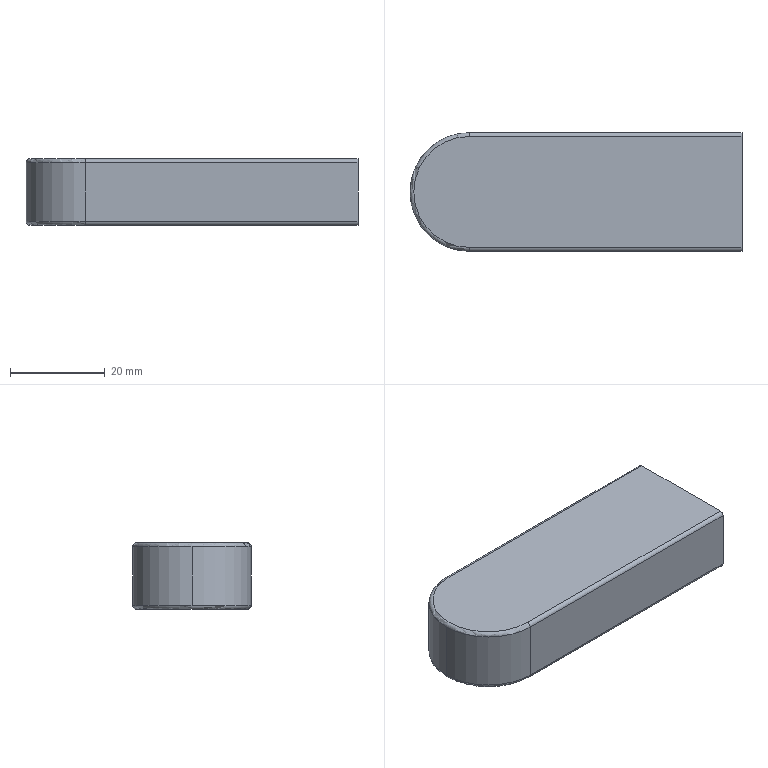Part | SolidWorks | features Extrusion 1, Fillet 1 | 1 solid | 13 faces | box 70 x 25 x 14 mm | volume 23519 mm3 | cylinder 6 | plane 5 | torus 2 | commonest cylinder face diameters 1.6 x4 25 x2
STEP:
#1=CARTESIAN_POINT('',(-9.,-12.5,13.2));
#2=VERTEX_POINT('',#1);
#3=CARTESIAN_POINT('',(-21.5,0.,13.2));
#4=VERTEX_POINT('',#3);
#5=CARTESIAN_POINT('',(-9.,0.,13.2));
#6=DIRECTION('',(0.,0.,-1.));
#7=DIRECTION('',(1.,0.,0.));
#8=AXIS2_PLACEMENT_3D('',#5,#6,#7);
#9=CIRCLE('',#8,12.5);
#10=EDGE_CURVE('',#2,#4,#9,.T.);
#11=ORIENTED_EDGE('',*,*,#10,.T.);
#12=CARTESIAN_POINT('',(-21.5,0.,0.8));
#13=VERTEX_POINT('',#12);
#14=CARTESIAN_POINT('',(-21.5,0.,14.));
#15=DIRECTION('',(0.,0.,-1.));
#16=VECTOR('',#15,1000.);
#17=LINE('',#14,#16);
#18=EDGE_CURVE('',#4,#13,#17,.T.);
#19=ORIENTED_EDGE('',*,*,#18,.T.);
#20=CARTESIAN_POINT('',(-9.,-12.5,0.8));
#21=VERTEX_POINT('',#20);
#22=CARTESIAN_POINT('',(-9.,0.,0.8));
#23=DIRECTION('',(0.,0.,1.));
#24=DIRECTION('',(1.,0.,0.));
#25=AXIS2_PLACEMENT_3D('',#22,#23,#24);
#26=CIRCLE('',#25,12.5);
#27=EDGE_CURVE('',#13,#21,#26,.T.);
#28=ORIENTED_EDGE('',*,*,#27,.T.);
#29=CARTESIAN_POINT('',(-9.,-12.5,14.));
#30=DIRECTION('',(0.,0.,-1.));
#31=VECTOR('',#30,1000.);
#32=LINE('',#29,#31);
#33=EDGE_CURVE('',#2,#21,#32,.T.);
#34=ORIENTED_EDGE('',*,*,#33,.F.);
#35=EDGE_LOOP('',(#11,#19,#28,#34));
#36=FACE_OUTER_BOUND('',#35,.T.);
#37=CARTESIAN_POINT('',(-9.,0.,14.));
#38=DIRECTION('',(0.,0.,-1.));
#39=DIRECTION('',(-1.,0.,0.));
#40=AXIS2_PLACEMENT_3D('',#37,#38,#39);
#41=CYLINDRICAL_SURFACE('',#40,12.5);
#42=ADVANCED_FACE('',(#36),#41,.T.);
#43=CARTESIAN_POINT('',(48.5,-11.7,14.));
#44=VERTEX_POINT('',#43);
#45=CARTESIAN_POINT('',(48.5,11.7,14.));
#46=VERTEX_POINT('',#45);
#47=CARTESIAN_POINT('',(48.5,12.5,14.));
#48=DIRECTION('',(0.,1.,0.));
#49=VECTOR('',#48,1000.);
#50=LINE('',#47,#49);
#51=EDGE_CURVE('',#44,#46,#50,.T.);
#52=ORIENTED_EDGE('',*,*,#51,.F.);
#53=CARTESIAN_POINT('',(48.5,-12.5,13.2));
#54=VERTEX_POINT('',#53);
#55=CARTESIAN_POINT('',(48.5,-11.7,13.2));
#56=DIRECTION('',(1.,0.,0.));
#57=DIRECTION('',(0.,0.,1.));
#58=AXIS2_PLACEMENT_3D('',#55,#56,#57);
#59=CIRCLE('',#58,0.8);
#60=EDGE_CURVE('',#44,#54,#59,.T.);
#61=ORIENTED_EDGE('',*,*,#60,.T.);
#62=CARTESIAN_POINT('',(48.5,-12.5,0.8));
#63=VERTEX_POINT('',#62);
#64=CARTESIAN_POINT('',(48.5,-12.5,14.));
#65=DIRECTION('',(0.,0.,-1.));
#66=VECTOR('',#65,1000.);
#67=LINE('',#64,#66);
#68=EDGE_CURVE('',#54,#63,#67,.T.);
#69=ORIENTED_EDGE('',*,*,#68,.T.);
#70=CARTESIAN_POINT('',(48.5,-11.7,0.));
#71=VERTEX_POINT('',#70);
#72=CARTESIAN_POINT('',(48.5,-11.7,0.8));
#73=DIRECTION('',(1.,0.,0.));
#74=DIRECTION('',(0.,0.,1.));
#75=AXIS2_PLACEMENT_3D('',#72,#73,#74);
#76=CIRCLE('',#75,0.8);
#77=EDGE_CURVE('',#63,#71,#76,.T.);
#78=ORIENTED_EDGE('',*,*,#77,.T.);
#79=CARTESIAN_POINT('',(48.5,11.7,0.));
#80=VERTEX_POINT('',#79);
#81=CARTESIAN_POINT('',(48.5,12.5,0.));
#82=DIRECTION('',(0.,1.,0.));
#83=VECTOR('',#82,1000.);
#84=LINE('',#81,#83);
#85=EDGE_CURVE('',#71,#80,#84,.T.);
#86=ORIENTED_EDGE('',*,*,#85,.T.);
#87=CARTESIAN_POINT('',(48.5,12.5,0.8));
#88=VERTEX_POINT('',#87);
#89=CARTESIAN_POINT('',(48.5,11.7,0.8));
#90=DIRECTION('',(1.,0.,0.));
#91=DIRECTION('',(0.,0.,1.));
#92=AXIS2_PLACEMENT_3D('',#89,#90,#91);
#93=CIRCLE('',#92,0.8);
#94=EDGE_CURVE('',#80,#88,#93,.T.);
#95=ORIENTED_EDGE('',*,*,#94,.T.);
#96=CARTESIAN_POINT('',(48.5,12.5,13.2));
#97=VERTEX_POINT('',#96);
#98=CARTESIAN_POINT('',(48.5,12.5,14.));
#99=DIRECTION('',(0.,0.,-1.));
#100=VECTOR('',#99,1000.);
#101=LINE('',#98,#100);
#102=EDGE_CURVE('',#97,#88,#101,.T.);
#103=ORIENTED_EDGE('',*,*,#102,.F.);
#104=CARTESIAN_POINT('',(48.5,11.7,13.2));
#105=DIRECTION('',(1.,0.,0.));
#106=DIRECTION('',(0.,0.,1.));
#107=AXIS2_PLACEMENT_3D('',#104,#105,#106);
#108=CIRCLE('',#107,0.8);
#109=EDGE_CURVE('',#97,#46,#108,.T.);
#110=ORIENTED_EDGE('',*,*,#109,.T.);
#111=EDGE_LOOP('',(#52,#61,#69,#78,#86,#95,#103,#110));
#112=FACE_OUTER_BOUND('',#111,.T.);
#113=CARTESIAN_POINT('',(48.5,12.5,14.));
#114=DIRECTION('',(-1.,0.,0.));
#115=DIRECTION('',(0.,0.,1.));
#116=AXIS2_PLACEMENT_3D('',#113,#114,#115);
#117=PLANE('',#116);
#118=ADVANCED_FACE('',(#112),#117,.F.);
#119=CARTESIAN_POINT('',(-9.,12.5,13.2));
#120=VERTEX_POINT('',#119);
#121=CARTESIAN_POINT('',(-9.,12.5,0.8));
#122=VERTEX_POINT('',#121);
#123=CARTESIAN_POINT('',(-9.,12.5,14.));
#124=DIRECTION('',(0.,0.,-1.));
#125=VECTOR('',#124,1000.);
#126=LINE('',#123,#125);
#127=EDGE_CURVE('',#120,#122,#126,.T.);
#128=ORIENTED_EDGE('',*,*,#127,.F.);
#129=CARTESIAN_POINT('',(48.5,12.5,13.2));
#130=DIRECTION('',(1.,0.,0.));
#131=VECTOR('',#130,1000.);
#132=LINE('',#129,#131);
#133=EDGE_CURVE('',#120,#97,#132,.T.);
#134=ORIENTED_EDGE('',*,*,#133,.T.);
#135=ORIENTED_EDGE('',*,*,#102,.T.);
#136=CARTESIAN_POINT('',(-9.,12.5,0.8));
#137=DIRECTION('',(-1.,0.,0.));
#138=VECTOR('',#137,1000.);
#139=LINE('',#136,#138);
#140=EDGE_CURVE('',#88,#122,#139,.T.);
#141=ORIENTED_EDGE('',*,*,#140,.T.);
#142=EDGE_LOOP('',(#128,#134,#135,#141));
#143=FACE_OUTER_BOUND('',#142,.T.);
#144=CARTESIAN_POINT('',(-9.,12.5,14.));
#145=DIRECTION('',(0.,-1.,0.));
#146=DIRECTION('',(0.,0.,-1.));
#147=AXIS2_PLACEMENT_3D('',#144,#145,#146);
#148=PLANE('',#147);
#149=ADVANCED_FACE('',(#143),#148,.F.);
#150=ORIENTED_EDGE('',*,*,#18,.F.);
#151=CARTESIAN_POINT('',(-9.,0.,13.2));
#152=DIRECTION('',(0.,0.,-1.));
#153=DIRECTION('',(1.,0.,0.));
#154=AXIS2_PLACEMENT_3D('',#151,#152,#153);
#155=CIRCLE('',#154,12.5);
#156=EDGE_CURVE('',#4,#120,#155,.T.);
#157=ORIENTED_EDGE('',*,*,#156,.T.);
#158=ORIENTED_EDGE('',*,*,#127,.T.);
#159=CARTESIAN_POINT('',(-9.,0.,0.8));
#160=DIRECTION('',(0.,0.,1.));
#161=DIRECTION('',(1.,0.,0.));
#162=AXIS2_PLACEMENT_3D('',#159,#160,#161);
#163=CIRCLE('',#162,12.5);
#164=EDGE_CURVE('',#122,#13,#163,.T.);
#165=ORIENTED_EDGE('',*,*,#164,.T.);
#166=EDGE_LOOP('',(#150,#157,#158,#165));
#167=FACE_OUTER_BOUND('',#166,.T.);
#168=CARTESIAN_POINT('',(-9.,0.,14.));
#169=DIRECTION('',(0.,0.,-1.));
#170=DIRECTION('',(-1.,0.,0.));
#171=AXIS2_PLACEMENT_3D('',#168,#169,#170);
#172=CYLINDRICAL_SURFACE('',#171,12.5);
#173=ADVANCED_FACE('',(#167),#172,.T.);
#174=ORIENTED_EDGE('',*,*,#68,.F.);
#175=CARTESIAN_POINT('',(-9.,-12.5,13.2));
#176=DIRECTION('',(-1.,0.,0.));
#177=VECTOR('',#176,1000.);
#178=LINE('',#175,#177);
#179=EDGE_CURVE('',#54,#2,#178,.T.);
#180=ORIENTED_EDGE('',*,*,#179,.T.);
#181=ORIENTED_EDGE('',*,*,#33,.T.);
#182=CARTESIAN_POINT('',(-9.,-12.5,0.8));
#183=DIRECTION('',(1.,0.,0.));
#184=VECTOR('',#183,1000.);
#185=LINE('',#182,#184);
#186=EDGE_CURVE('',#21,#63,#185,.T.);
#187=ORIENTED_EDGE('',*,*,#186,.T.);
#188=EDGE_LOOP('',(#174,#180,#181,#187));
#189=FACE_OUTER_BOUND('',#188,.T.);
#190=CARTESIAN_POINT('',(-9.,-12.5,14.));
#191=DIRECTION('',(0.,1.,0.));
#192=DIRECTION('',(0.,0.,1.));
#193=AXIS2_PLACEMENT_3D('',#190,#191,#192);
#194=PLANE('',#193);
#195=ADVANCED_FACE('',(#189),#194,.F.);
#196=CARTESIAN_POINT('',(-9.,11.7,14.));
#197=VERTEX_POINT('',#196);
#198=CARTESIAN_POINT('',(-9.,-11.7,14.));
#199=VERTEX_POINT('',#198);
#200=CARTESIAN_POINT('',(-9.,0.,14.));
#201=DIRECTION('',(0.,0.,1.));
#202=DIRECTION('',(1.,0.,0.));
#203=AXIS2_PLACEMENT_3D('',#200,#201,#202);
#204=CIRCLE('',#203,11.7);
#205=EDGE_CURVE('',#197,#199,#204,.T.);
#206=ORIENTED_EDGE('',*,*,#205,.T.);
#207=CARTESIAN_POINT('',(48.5,-11.7,14.));
#208=DIRECTION('',(1.,0.,0.));
#209=VECTOR('',#208,1000.);
#210=LINE('',#207,#209);
#211=EDGE_CURVE('',#199,#44,#210,.T.);
#212=ORIENTED_EDGE('',*,*,#211,.T.);
#213=ORIENTED_EDGE('',*,*,#51,.T.);
#214=CARTESIAN_POINT('',(-9.,11.7,14.));
#215=DIRECTION('',(-1.,0.,0.));
#216=VECTOR('',#215,1000.);
#217=LINE('',#214,#216);
#218=EDGE_CURVE('',#46,#197,#217,.T.);
#219=ORIENTED_EDGE('',*,*,#218,.T.);
#220=EDGE_LOOP('',(#206,#212,#213,#219));
#221=FACE_OUTER_BOUND('',#220,.T.);
#222=CARTESIAN_POINT('',(-9.,0.,14.));
#223=DIRECTION('',(0.,0.,1.));
#224=DIRECTION('',(1.,0.,0.));
#225=AXIS2_PLACEMENT_3D('',#222,#223,#224);
#226=PLANE('',#225);
#227=ADVANCED_FACE('',(#221),#226,.T.);
#228=CARTESIAN_POINT('',(-9.,-11.7,0.));
#229=VERTEX_POINT('',#228);
#230=CARTESIAN_POINT('',(-9.,11.7,0.));
#231=VERTEX_POINT('',#230);
#232=CARTESIAN_POINT('',(-9.,0.,0.));
#233=DIRECTION('',(0.,0.,-1.));
#234=DIRECTION('',(1.,0.,0.));
#235=AXIS2_PLACEMENT_3D('',#232,#233,#234);
#236=CIRCLE('',#235,11.7);
#237=EDGE_CURVE('',#229,#231,#236,.T.);
#238=ORIENTED_EDGE('',*,*,#237,.T.);
#239=CARTESIAN_POINT('',(-9.,11.7,0.));
#240=DIRECTION('',(1.,0.,0.));
#241=VECTOR('',#240,1000.);
#242=LINE('',#239,#241);
#243=EDGE_CURVE('',#231,#80,#242,.T.);
#244=ORIENTED_EDGE('',*,*,#243,.T.);
#245=ORIENTED_EDGE('',*,*,#85,.F.);
#246=CARTESIAN_POINT('',(-9.,-11.7,0.));
#247=DIRECTION('',(-1.,0.,0.));
#248=VECTOR('',#247,1000.);
#249=LINE('',#246,#248);
#250=EDGE_CURVE('',#71,#229,#249,.T.);
#251=ORIENTED_EDGE('',*,*,#250,.T.);
#252=EDGE_LOOP('',(#238,#244,#245,#251));
#253=FACE_OUTER_BOUND('',#252,.T.);
#254=CARTESIAN_POINT('',(-9.,0.,0.));
#255=DIRECTION('',(0.,0.,1.));
#256=DIRECTION('',(1.,0.,0.));
#257=AXIS2_PLACEMENT_3D('',#254,#255,#256);
#258=PLANE('',#257);
#259=ADVANCED_FACE('',(#253),#258,.F.);
#260=ORIENTED_EDGE('',*,*,#109,.F.);
#261=ORIENTED_EDGE('',*,*,#133,.F.);
#262=CARTESIAN_POINT('',(-9.,11.7,13.2));
#263=DIRECTION('',(-1.,0.,0.));
#264=DIRECTION('',(0.,0.,1.));
#265=AXIS2_PLACEMENT_3D('',#262,#263,#264);
#266=CIRCLE('',#265,0.8);
#267=EDGE_CURVE('',#197,#120,#266,.T.);
#268=ORIENTED_EDGE('',*,*,#267,.F.);
#269=ORIENTED_EDGE('',*,*,#218,.F.);
#270=EDGE_LOOP('',(#260,#261,#268,#269));
#271=FACE_OUTER_BOUND('',#270,.T.);
#272=CARTESIAN_POINT('',(-9.,11.7,13.2));
#273=DIRECTION('',(1.,0.,0.));
#274=DIRECTION('',(0.,0.,-1.));
#275=AXIS2_PLACEMENT_3D('',#272,#273,#274);
#276=CYLINDRICAL_SURFACE('',#275,0.8);
#277=ADVANCED_FACE('',(#271),#276,.T.);
#278=ORIENTED_EDGE('',*,*,#267,.T.);
#279=ORIENTED_EDGE('',*,*,#156,.F.);
#280=ORIENTED_EDGE('',*,*,#10,.F.);
#281=CARTESIAN_POINT('',(-9.,-11.7,13.2));
#282=DIRECTION('',(1.,0.,0.));
#283=DIRECTION('',(0.,0.,-1.));
#284=AXIS2_PLACEMENT_3D('',#281,#282,#283);
#285=CIRCLE('',#284,0.8);
#286=EDGE_CURVE('',#199,#2,#285,.T.);
#287=ORIENTED_EDGE('',*,*,#286,.F.);
#288=ORIENTED_EDGE('',*,*,#205,.F.);
#289=EDGE_LOOP('',(#278,#279,#280,#287,#288));
#290=FACE_OUTER_BOUND('',#289,.T.);
#291=CARTESIAN_POINT('',(-9.,0.,13.2));
#292=DIRECTION('',(0.,0.,1.));
#293=DIRECTION('',(1.,0.,0.));
#294=AXIS2_PLACEMENT_3D('',#291,#292,#293);
#295=TOROIDAL_SURFACE('',#294,11.7,0.8);
#296=ADVANCED_FACE('',(#290),#295,.T.);
#297=ORIENTED_EDGE('',*,*,#286,.T.);
#298=ORIENTED_EDGE('',*,*,#179,.F.);
#299=ORIENTED_EDGE('',*,*,#60,.F.);
#300=ORIENTED_EDGE('',*,*,#211,.F.);
#301=EDGE_LOOP('',(#297,#298,#299,#300));
#302=FACE_OUTER_BOUND('',#301,.T.);
#303=CARTESIAN_POINT('',(-9.,-11.7,13.2));
#304=DIRECTION('',(-1.,0.,0.));
#305=DIRECTION('',(0.,0.,1.));
#306=AXIS2_PLACEMENT_3D('',#303,#304,#305);
#307=CYLINDRICAL_SURFACE('',#306,0.8);
#308=ADVANCED_FACE('',(#302),#307,.T.);
#309=ORIENTED_EDGE('',*,*,#77,.F.);
#310=ORIENTED_EDGE('',*,*,#186,.F.);
#311=CARTESIAN_POINT('',(-9.,-11.7,0.8));
#312=DIRECTION('',(-1.,0.,0.));
#313=DIRECTION('',(0.,0.,1.));
#314=AXIS2_PLACEMENT_3D('',#311,#312,#313);
#315=CIRCLE('',#314,0.8);
#316=EDGE_CURVE('',#229,#21,#315,.T.);
#317=ORIENTED_EDGE('',*,*,#316,.F.);
#318=ORIENTED_EDGE('',*,*,#250,.F.);
#319=EDGE_LOOP('',(#309,#310,#317,#318));
#320=FACE_OUTER_BOUND('',#319,.T.);
#321=CARTESIAN_POINT('',(-9.,-11.7,0.8));
#322=DIRECTION('',(1.,0.,0.));
#323=DIRECTION('',(0.,0.,-1.));
#324=AXIS2_PLACEMENT_3D('',#321,#322,#323);
#325=CYLINDRICAL_SURFACE('',#324,0.8);
#326=ADVANCED_FACE('',(#320),#325,.T.);
#327=ORIENTED_EDGE('',*,*,#316,.T.);
#328=ORIENTED_EDGE('',*,*,#27,.F.);
#329=ORIENTED_EDGE('',*,*,#164,.F.);
#330=CARTESIAN_POINT('',(-9.,11.7,0.8));
#331=DIRECTION('',(1.,0.,0.));
#332=DIRECTION('',(0.,0.,-1.));
#333=AXIS2_PLACEMENT_3D('',#330,#331,#332);
#334=CIRCLE('',#333,0.8);
#335=EDGE_CURVE('',#231,#122,#334,.T.);
#336=ORIENTED_EDGE('',*,*,#335,.F.);
#337=ORIENTED_EDGE('',*,*,#237,.F.);
#338=EDGE_LOOP('',(#327,#328,#329,#336,#337));
#339=FACE_OUTER_BOUND('',#338,.T.);
#340=CARTESIAN_POINT('',(-9.,0.,0.8));
#341=DIRECTION('',(0.,0.,1.));
#342=DIRECTION('',(1.,0.,0.));
#343=AXIS2_PLACEMENT_3D('',#340,#341,#342);
#344=TOROIDAL_SURFACE('',#343,11.7,0.8);
#345=ADVANCED_FACE('',(#339),#344,.T.);
#346=ORIENTED_EDGE('',*,*,#94,.F.);
#347=ORIENTED_EDGE('',*,*,#243,.F.);
#348=ORIENTED_EDGE('',*,*,#335,.T.);
#349=ORIENTED_EDGE('',*,*,#140,.F.);
#350=EDGE_LOOP('',(#346,#347,#348,#349));
#351=FACE_OUTER_BOUND('',#350,.T.);
#352=CARTESIAN_POINT('',(-9.,11.7,0.8));
#353=DIRECTION('',(-1.,0.,0.));
#354=DIRECTION('',(0.,0.,1.));
#355=AXIS2_PLACEMENT_3D('',#352,#353,#354);
#356=CYLINDRICAL_SURFACE('',#355,0.8);
#357=ADVANCED_FACE('',(#351),#356,.T.);
#358=CLOSED_SHELL('',(#42,#118,#149,#173,#195,#227,#259,#277,#296,#308,#326,#345,#357));
#359=MANIFOLD_SOLID_BREP('',#358);
#360=CARTESIAN_POINT('',(0.,0.,0.));
#361=DIRECTION('',(0.,0.,1.));
#362=DIRECTION('',(1.,0.,0.));
#363=AXIS2_PLACEMENT_3D('',#360,#361,#362);
#364=(LENGTH_UNIT()NAMED_UNIT(*)SI_UNIT(.MILLI.,.METRE.));
#365=UNCERTAINTY_MEASURE_WITH_UNIT(LENGTH_MEASURE(0.00001),#364,'','');
#366=(NAMED_UNIT(*)PLANE_ANGLE_UNIT()SI_UNIT($,.RADIAN.));
#367=(NAMED_UNIT(*)SI_UNIT($,.STERADIAN.)SOLID_ANGLE_UNIT());
#368=(GEOMETRIC_REPRESENTATION_CONTEXT(3)GLOBAL_UNCERTAINTY_ASSIGNED_CONTEXT((#365))GLOBAL_UNIT_ASSIGNED_CONTEXT((#364,#366,#367))REPRESENTATION_CONTEXT('',''));
#369=ADVANCED_BREP_SHAPE_REPRESENTATION('',(#359,#363),#368);